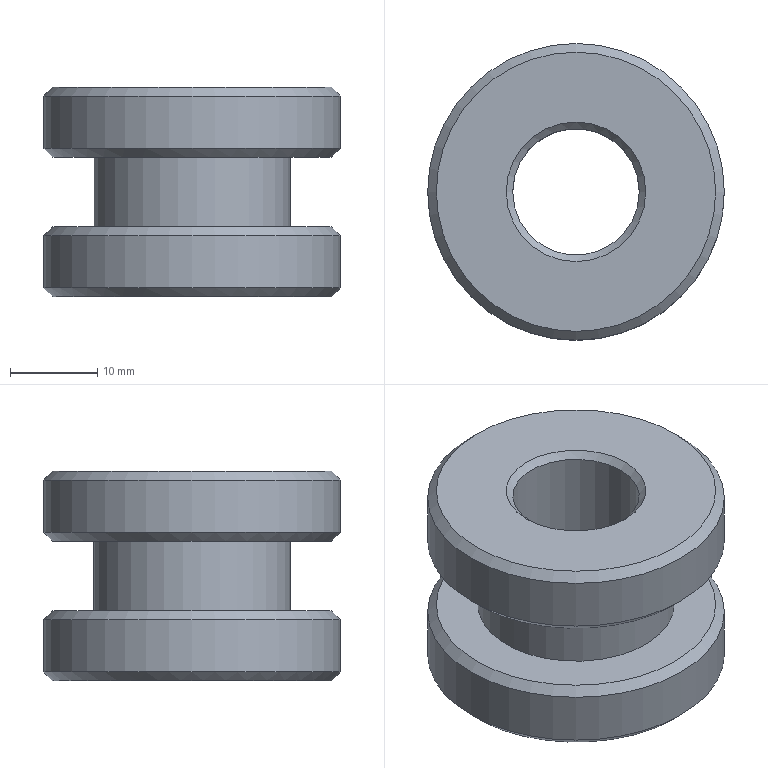Part | STEP file | YBQDJ-QD-9 | 1 solid | 14 faces | box 34 x 34 x 24 mm | volume 13509 mm3 | cone 6 | cylinder 4 | plane 4 | commonest cylinder face diameters 34 x2 14.5 x1 22.5 x1
STEP:
#1=CARTESIAN_POINT('',(0.,0.,0.));
#2=DIRECTION('',(0.,0.,1.));
#3=DIRECTION('',(1.,0.,0.));
#4=AXIS2_PLACEMENT_3D('',#1,#2,#3);
#5=CARTESIAN_POINT('',(-332.75,-195.,209.25));
#6=VERTEX_POINT('',#5);
#7=CARTESIAN_POINT('',(-340.,-195.,209.25));
#8=DIRECTION('',(0.,0.,-1.));
#9=DIRECTION('',(1.,0.,0.));
#10=AXIS2_PLACEMENT_3D('',#7,#8,#9);
#11=CIRCLE('',#10,7.25);
#12=CARTESIAN_POINT('',(-340.,-195.,232.5));
#13=DIRECTION('',(0.,0.,-1.));
#14=DIRECTION('',(-1.,0.,0.));
#15=AXIS2_PLACEMENT_3D('',#12,#13,#14);
#16=CYLINDRICAL_SURFACE('',#15,7.25);
#17=CARTESIAN_POINT('',(3.142,23.25));
#18=DIRECTION('',(1.,0.));
#19=VECTOR('',#18,1.);
#20=LINE('',#17,#19);
#21=(GEOMETRIC_REPRESENTATION_CONTEXT(2)PARAMETRIC_REPRESENTATION_CONTEXT()REPRESENTATION_CONTEXT('',''));
#22=DEFINITIONAL_REPRESENTATION('',(#20),#21);
#23=PCURVE('',#16,#22);
#24=CARTESIAN_POINT('',(-340.,-195.,209.25));
#25=DIRECTION('',(0.,0.,-1.));
#26=DIRECTION('',(-1.,0.,0.));
#27=AXIS2_PLACEMENT_3D('',#24,#25,#26);
#28=CONICAL_SURFACE('',#27,7.25,0.7854);
#29=CARTESIAN_POINT('',(3.142,0.));
#30=DIRECTION('',(1.,0.));
#31=VECTOR('',#30,1.);
#32=LINE('',#29,#31);
#33=(GEOMETRIC_REPRESENTATION_CONTEXT(2)PARAMETRIC_REPRESENTATION_CONTEXT()REPRESENTATION_CONTEXT('',''));
#34=DEFINITIONAL_REPRESENTATION('',(#32),#33);
#35=PCURVE('',#28,#34);
#36=SURFACE_CURVE('',#11,(#23,#35),.PCURVE_S1.);
#37=EDGE_CURVE('',#6,#6,#36,.T.);
#38=ORIENTED_EDGE('',*,*,#37,.F.);
#39=CARTESIAN_POINT('',(-332.75,-195.,231.75));
#40=VERTEX_POINT('',#39);
#41=CARTESIAN_POINT('',(-332.75,-195.,231.75));
#42=CARTESIAN_POINT('',(-332.75,-195.,209.25));
#43=B_SPLINE_CURVE_WITH_KNOTS('',1,(#41,#42),.UNSPECIFIED.,.F.,.F.,(2,2),(0.75,23.25),.PIECEWISE_BEZIER_KNOTS.);
#44=CARTESIAN_POINT('',(3.142,0.));
#45=DIRECTION('',(0.,1.));
#46=VECTOR('',#45,1.);
#47=LINE('',#44,#46);
#48=(GEOMETRIC_REPRESENTATION_CONTEXT(2)PARAMETRIC_REPRESENTATION_CONTEXT()REPRESENTATION_CONTEXT('',''));
#49=DEFINITIONAL_REPRESENTATION('',(#47),#48);
#50=PCURVE('',#16,#49);
#51=CARTESIAN_POINT('',(9.425,0.));
#52=DIRECTION('',(0.,1.));
#53=VECTOR('',#52,1.);
#54=LINE('',#51,#53);
#55=(GEOMETRIC_REPRESENTATION_CONTEXT(2)PARAMETRIC_REPRESENTATION_CONTEXT()REPRESENTATION_CONTEXT('',''));
#56=DEFINITIONAL_REPRESENTATION('',(#54),#55);
#57=PCURVE('',#16,#56);
#58=SEAM_CURVE('',#43,(#50,#57),.PCURVE_S1.);
#59=EDGE_CURVE('',#40,#6,#58,.T.);
#60=ORIENTED_EDGE('',*,*,#59,.F.);
#61=CARTESIAN_POINT('',(-340.,-195.,231.75));
#62=DIRECTION('',(0.,0.,1.));
#63=DIRECTION('',(1.,0.,0.));
#64=AXIS2_PLACEMENT_3D('',#61,#62,#63);
#65=CIRCLE('',#64,7.25);
#66=CARTESIAN_POINT('',(9.425,0.75));
#67=DIRECTION('',(-1.,0.));
#68=VECTOR('',#67,1.);
#69=LINE('',#66,#68);
#70=(GEOMETRIC_REPRESENTATION_CONTEXT(2)PARAMETRIC_REPRESENTATION_CONTEXT()REPRESENTATION_CONTEXT('',''));
#71=DEFINITIONAL_REPRESENTATION('',(#69),#70);
#72=PCURVE('',#16,#71);
#73=CARTESIAN_POINT('',(-340.,-195.,231.75));
#74=DIRECTION('',(0.,0.,1.));
#75=DIRECTION('',(1.,0.,0.));
#76=AXIS2_PLACEMENT_3D('',#73,#74,#75);
#77=CONICAL_SURFACE('',#76,7.25,0.7854);
#78=CARTESIAN_POINT('',(0.,0.));
#79=DIRECTION('',(1.,0.));
#80=VECTOR('',#79,1.);
#81=LINE('',#78,#80);
#82=(GEOMETRIC_REPRESENTATION_CONTEXT(2)PARAMETRIC_REPRESENTATION_CONTEXT()REPRESENTATION_CONTEXT('',''));
#83=DEFINITIONAL_REPRESENTATION('',(#81),#82);
#84=PCURVE('',#77,#83);
#85=SURFACE_CURVE('',#65,(#72,#84),.PCURVE_S1.);
#86=EDGE_CURVE('',#40,#40,#85,.T.);
#87=ORIENTED_EDGE('',*,*,#86,.F.);
#88=ORIENTED_EDGE('',*,*,#59,.T.);
#89=EDGE_LOOP('',(#38,#60,#87,#88));
#90=FACE_BOUND('',#89,.F.);
#91=ADVANCED_FACE('',(#90),#16,.F.);
#92=CARTESIAN_POINT('',(-323.,-195.,225.5));
#93=VERTEX_POINT('',#92);
#94=CARTESIAN_POINT('',(-357.,-195.,225.5));
#95=VERTEX_POINT('',#94);
#96=CARTESIAN_POINT('',(-340.,-195.,225.5));
#97=DIRECTION('',(0.,0.,1.));
#98=DIRECTION('',(1.,0.,0.));
#99=AXIS2_PLACEMENT_3D('',#96,#97,#98);
#100=CIRCLE('',#99,17.);
#101=CARTESIAN_POINT('',(-340.,-195.,232.5));
#102=DIRECTION('',(0.,0.,-1.));
#103=DIRECTION('',(-1.,0.,0.));
#104=AXIS2_PLACEMENT_3D('',#101,#102,#103);
#105=CYLINDRICAL_SURFACE('',#104,17.);
#106=CARTESIAN_POINT('',(3.142,7.));
#107=DIRECTION('',(-1.,0.));
#108=VECTOR('',#107,1.);
#109=LINE('',#106,#108);
#110=(GEOMETRIC_REPRESENTATION_CONTEXT(2)PARAMETRIC_REPRESENTATION_CONTEXT()REPRESENTATION_CONTEXT('',''));
#111=DEFINITIONAL_REPRESENTATION('',(#109),#110);
#112=PCURVE('',#105,#111);
#113=CARTESIAN_POINT('',(-340.,-195.,225.5));
#114=DIRECTION('',(0.,0.,1.));
#115=DIRECTION('',(1.,0.,0.));
#116=AXIS2_PLACEMENT_3D('',#113,#114,#115);
#117=CONICAL_SURFACE('',#116,17.,0.7854);
#118=CARTESIAN_POINT('',(0.,0.));
#119=DIRECTION('',(1.,0.));
#120=VECTOR('',#119,1.);
#121=LINE('',#118,#120);
#122=(GEOMETRIC_REPRESENTATION_CONTEXT(2)PARAMETRIC_REPRESENTATION_CONTEXT()REPRESENTATION_CONTEXT('',''));
#123=DEFINITIONAL_REPRESENTATION('',(#121),#122);
#124=PCURVE('',#117,#123);
#125=SURFACE_CURVE('',#100,(#112,#124),.PCURVE_S1.);
#126=EDGE_CURVE('',#93,#95,#125,.T.);
#127=ORIENTED_EDGE('',*,*,#126,.T.);
#128=CARTESIAN_POINT('',(-357.,-195.,231.5));
#129=VERTEX_POINT('',#128);
#130=CARTESIAN_POINT('',(-357.,-195.,231.5));
#131=CARTESIAN_POINT('',(-357.,-195.,225.5));
#132=B_SPLINE_CURVE_WITH_KNOTS('',1,(#130,#131),.UNSPECIFIED.,.F.,.F.,(2,2),(1.,7.),.PIECEWISE_BEZIER_KNOTS.);
#133=CARTESIAN_POINT('',(0.,0.));
#134=DIRECTION('',(0.,1.));
#135=VECTOR('',#134,1.);
#136=LINE('',#133,#135);
#137=(GEOMETRIC_REPRESENTATION_CONTEXT(2)PARAMETRIC_REPRESENTATION_CONTEXT()REPRESENTATION_CONTEXT('',''));
#138=DEFINITIONAL_REPRESENTATION('',(#136),#137);
#139=PCURVE('',#105,#138);
#140=CARTESIAN_POINT('',(6.283,0.));
#141=DIRECTION('',(0.,1.));
#142=VECTOR('',#141,1.);
#143=LINE('',#140,#142);
#144=(GEOMETRIC_REPRESENTATION_CONTEXT(2)PARAMETRIC_REPRESENTATION_CONTEXT()REPRESENTATION_CONTEXT('',''));
#145=DEFINITIONAL_REPRESENTATION('',(#143),#144);
#146=PCURVE('',#105,#145);
#147=SEAM_CURVE('',#132,(#139,#146),.PCURVE_S1.);
#148=EDGE_CURVE('',#129,#95,#147,.T.);
#149=ORIENTED_EDGE('',*,*,#148,.F.);
#150=CARTESIAN_POINT('',(-340.,-195.,231.5));
#151=DIRECTION('',(0.,0.,-1.));
#152=DIRECTION('',(-1.,0.,0.));
#153=AXIS2_PLACEMENT_3D('',#150,#151,#152);
#154=CIRCLE('',#153,17.);
#155=CARTESIAN_POINT('',(0.,1.));
#156=DIRECTION('',(1.,0.));
#157=VECTOR('',#156,1.);
#158=LINE('',#155,#157);
#159=(GEOMETRIC_REPRESENTATION_CONTEXT(2)PARAMETRIC_REPRESENTATION_CONTEXT()REPRESENTATION_CONTEXT('',''));
#160=DEFINITIONAL_REPRESENTATION('',(#158),#159);
#161=PCURVE('',#105,#160);
#162=CARTESIAN_POINT('',(-340.,-195.,232.5));
#163=DIRECTION('',(0.,0.,-1.));
#164=DIRECTION('',(-1.,0.,0.));
#165=AXIS2_PLACEMENT_3D('',#162,#163,#164);
#166=CONICAL_SURFACE('',#165,16.,0.7854);
#167=CARTESIAN_POINT('',(0.,1.));
#168=DIRECTION('',(1.,0.));
#169=VECTOR('',#168,1.);
#170=LINE('',#167,#169);
#171=(GEOMETRIC_REPRESENTATION_CONTEXT(2)PARAMETRIC_REPRESENTATION_CONTEXT()REPRESENTATION_CONTEXT('',''));
#172=DEFINITIONAL_REPRESENTATION('',(#170),#171);
#173=PCURVE('',#166,#172);
#174=SURFACE_CURVE('',#154,(#161,#173),.PCURVE_S1.);
#175=EDGE_CURVE('',#129,#129,#174,.T.);
#176=ORIENTED_EDGE('',*,*,#175,.T.);
#177=ORIENTED_EDGE('',*,*,#148,.T.);
#178=CARTESIAN_POINT('',(-340.,-195.,225.5));
#179=DIRECTION('',(0.,0.,1.));
#180=DIRECTION('',(1.,0.,0.));
#181=AXIS2_PLACEMENT_3D('',#178,#179,#180);
#182=CIRCLE('',#181,17.);
#183=CARTESIAN_POINT('',(9.425,7.));
#184=DIRECTION('',(-1.,0.));
#185=VECTOR('',#184,1.);
#186=LINE('',#183,#185);
#187=(GEOMETRIC_REPRESENTATION_CONTEXT(2)PARAMETRIC_REPRESENTATION_CONTEXT()REPRESENTATION_CONTEXT('',''));
#188=DEFINITIONAL_REPRESENTATION('',(#186),#187);
#189=PCURVE('',#105,#188);
#190=CARTESIAN_POINT('',(0.,0.));
#191=DIRECTION('',(1.,0.));
#192=VECTOR('',#191,1.);
#193=LINE('',#190,#192);
#194=(GEOMETRIC_REPRESENTATION_CONTEXT(2)PARAMETRIC_REPRESENTATION_CONTEXT()REPRESENTATION_CONTEXT('',''));
#195=DEFINITIONAL_REPRESENTATION('',(#193),#194);
#196=PCURVE('',#117,#195);
#197=SURFACE_CURVE('',#182,(#189,#196),.PCURVE_S1.);
#198=EDGE_CURVE('',#95,#93,#197,.T.);
#199=ORIENTED_EDGE('',*,*,#198,.T.);
#200=EDGE_LOOP('',(#127,#149,#176,#177,#199));
#201=FACE_BOUND('',#200,.T.);
#202=ADVANCED_FACE('',(#201),#105,.T.);
#203=CARTESIAN_POINT('',(-324.,-195.,232.5));
#204=VERTEX_POINT('',#203);
#205=CARTESIAN_POINT('',(-356.,-195.,232.5));
#206=VERTEX_POINT('',#205);
#207=CARTESIAN_POINT('',(-340.,-195.,232.5));
#208=DIRECTION('',(0.,0.,1.));
#209=DIRECTION('',(1.,0.,0.));
#210=AXIS2_PLACEMENT_3D('',#207,#208,#209);
#211=CIRCLE('',#210,16.);
#212=CARTESIAN_POINT('',(-340.,-195.,232.5));
#213=DIRECTION('',(0.,0.,1.));
#214=DIRECTION('',(1.,0.,0.));
#215=AXIS2_PLACEMENT_3D('',#212,#213,#214);
#216=PLANE('',#215);
#217=CARTESIAN_POINT('',(0.,0.));
#218=DIRECTION('',(1.,0.));
#219=AXIS2_PLACEMENT_2D('',#217,#218);
#220=CIRCLE('',#219,16.);
#221=(GEOMETRIC_REPRESENTATION_CONTEXT(2)PARAMETRIC_REPRESENTATION_CONTEXT()REPRESENTATION_CONTEXT('',''));
#222=DEFINITIONAL_REPRESENTATION('',(#220),#221);
#223=PCURVE('',#216,#222);
#224=CARTESIAN_POINT('',(3.142,0.));
#225=DIRECTION('',(-1.,0.));
#226=VECTOR('',#225,1.);
#227=LINE('',#224,#226);
#228=(GEOMETRIC_REPRESENTATION_CONTEXT(2)PARAMETRIC_REPRESENTATION_CONTEXT()REPRESENTATION_CONTEXT('',''));
#229=DEFINITIONAL_REPRESENTATION('',(#227),#228);
#230=PCURVE('',#166,#229);
#231=SURFACE_CURVE('',#211,(#223,#230),.PCURVE_S1.);
#232=EDGE_CURVE('',#204,#206,#231,.T.);
#233=ORIENTED_EDGE('',*,*,#232,.T.);
#234=CARTESIAN_POINT('',(-340.,-195.,232.5));
#235=DIRECTION('',(0.,0.,1.));
#236=DIRECTION('',(1.,0.,0.));
#237=AXIS2_PLACEMENT_3D('',#234,#235,#236);
#238=CIRCLE('',#237,16.);
#239=CARTESIAN_POINT('',(0.,0.));
#240=DIRECTION('',(1.,0.));
#241=AXIS2_PLACEMENT_2D('',#239,#240);
#242=CIRCLE('',#241,16.);
#243=(GEOMETRIC_REPRESENTATION_CONTEXT(2)PARAMETRIC_REPRESENTATION_CONTEXT()REPRESENTATION_CONTEXT('',''));
#244=DEFINITIONAL_REPRESENTATION('',(#242),#243);
#245=PCURVE('',#216,#244);
#246=CARTESIAN_POINT('',(9.425,0.));
#247=DIRECTION('',(-1.,0.));
#248=VECTOR('',#247,1.);
#249=LINE('',#246,#248);
#250=(GEOMETRIC_REPRESENTATION_CONTEXT(2)PARAMETRIC_REPRESENTATION_CONTEXT()REPRESENTATION_CONTEXT('',''));
#251=DEFINITIONAL_REPRESENTATION('',(#249),#250);
#252=PCURVE('',#166,#251);
#253=SURFACE_CURVE('',#238,(#245,#252),.PCURVE_S1.);
#254=EDGE_CURVE('',#206,#204,#253,.T.);
#255=ORIENTED_EDGE('',*,*,#254,.T.);
#256=EDGE_LOOP('',(#233,#255));
#257=FACE_BOUND('',#256,.T.);
#258=CARTESIAN_POINT('',(-332.,-195.,232.5));
#259=VERTEX_POINT('',#258);
#260=CARTESIAN_POINT('',(-340.,-195.,232.5));
#261=DIRECTION('',(0.,0.,-1.));
#262=DIRECTION('',(1.,0.,0.));
#263=AXIS2_PLACEMENT_3D('',#260,#261,#262);
#264=CIRCLE('',#263,8.);
#265=CARTESIAN_POINT('',(8.,0.));
#266=CARTESIAN_POINT('',(8.,-13.856));
#267=CARTESIAN_POINT('',(-4.,-6.928));
#268=CARTESIAN_POINT('',(-16.,0.));
#269=CARTESIAN_POINT('',(-4.,6.928));
#270=CARTESIAN_POINT('',(8.,13.856));
#271=CARTESIAN_POINT('',(8.,0.));
#272=(BOUNDED_CURVE()B_SPLINE_CURVE(2,(#265,#266,#267,#268,#269,#270,#271),.UNSPECIFIED.,.T.,.F.)B_SPLINE_CURVE_WITH_KNOTS((1,2,2,2,2,1),(-2.094,0.,2.094,4.189,6.283,8.378),.UNSPECIFIED.)CURVE()GEOMETRIC_REPRESENTATION_ITEM()RATIONAL_B_SPLINE_CURVE((1.,0.5,1.,0.5,1.,0.5,1.))REPRESENTATION_ITEM(''));
#273=(GEOMETRIC_REPRESENTATION_CONTEXT(2)PARAMETRIC_REPRESENTATION_CONTEXT()REPRESENTATION_CONTEXT('',''));
#274=DEFINITIONAL_REPRESENTATION('',(#272),#273);
#275=PCURVE('',#216,#274);
#276=CARTESIAN_POINT('',(6.283,0.75));
#277=DIRECTION('',(-1.,0.));
#278=VECTOR('',#277,1.);
#279=LINE('',#276,#278);
#280=(GEOMETRIC_REPRESENTATION_CONTEXT(2)PARAMETRIC_REPRESENTATION_CONTEXT()REPRESENTATION_CONTEXT('',''));
#281=DEFINITIONAL_REPRESENTATION('',(#279),#280);
#282=PCURVE('',#77,#281);
#283=SURFACE_CURVE('',#264,(#275,#282),.PCURVE_S1.);
#284=EDGE_CURVE('',#259,#259,#283,.T.);
#285=ORIENTED_EDGE('',*,*,#284,.T.);
#286=EDGE_LOOP('',(#285));
#287=FACE_BOUND('',#286,.T.);
#288=ADVANCED_FACE('',(#257,#287),#216,.T.);
#289=CARTESIAN_POINT('',(-324.,-195.,224.5));
#290=VERTEX_POINT('',#289);
#291=CARTESIAN_POINT('',(-340.,-195.,224.5));
#292=DIRECTION('',(0.,0.,-1.));
#293=DIRECTION('',(1.,0.,0.));
#294=AXIS2_PLACEMENT_3D('',#291,#292,#293);
#295=CIRCLE('',#294,16.);
#296=CARTESIAN_POINT('',(-340.,-195.,224.5));
#297=DIRECTION('',(0.,0.,1.));
#298=DIRECTION('',(1.,0.,0.));
#299=AXIS2_PLACEMENT_3D('',#296,#297,#298);
#300=PLANE('',#299);
#301=CARTESIAN_POINT('',(16.,0.));
#302=CARTESIAN_POINT('',(16.,-27.713));
#303=CARTESIAN_POINT('',(-8.,-13.856));
#304=CARTESIAN_POINT('',(-32.,0.));
#305=CARTESIAN_POINT('',(-8.,13.856));
#306=CARTESIAN_POINT('',(16.,27.713));
#307=CARTESIAN_POINT('',(16.,0.));
#308=(BOUNDED_CURVE()B_SPLINE_CURVE(2,(#301,#302,#303,#304,#305,#306,#307),.UNSPECIFIED.,.T.,.F.)B_SPLINE_CURVE_WITH_KNOTS((1,2,2,2,2,1),(-2.094,0.,2.094,4.189,6.283,8.378),.UNSPECIFIED.)CURVE()GEOMETRIC_REPRESENTATION_ITEM()RATIONAL_B_SPLINE_CURVE((1.,0.5,1.,0.5,1.,0.5,1.))REPRESENTATION_ITEM(''));
#309=(GEOMETRIC_REPRESENTATION_CONTEXT(2)PARAMETRIC_REPRESENTATION_CONTEXT()REPRESENTATION_CONTEXT('',''));
#310=DEFINITIONAL_REPRESENTATION('',(#308),#309);
#311=PCURVE('',#300,#310);
#312=CARTESIAN_POINT('',(6.283,-1.));
#313=DIRECTION('',(-1.,0.));
#314=VECTOR('',#313,1.);
#315=LINE('',#312,#314);
#316=(GEOMETRIC_REPRESENTATION_CONTEXT(2)PARAMETRIC_REPRESENTATION_CONTEXT()REPRESENTATION_CONTEXT('',''));
#317=DEFINITIONAL_REPRESENTATION('',(#315),#316);
#318=PCURVE('',#117,#317);
#319=SURFACE_CURVE('',#295,(#311,#318),.PCURVE_S1.);
#320=EDGE_CURVE('',#290,#290,#319,.T.);
#321=ORIENTED_EDGE('',*,*,#320,.T.);
#322=EDGE_LOOP('',(#321));
#323=FACE_BOUND('',#322,.T.);
#324=CARTESIAN_POINT('',(-328.75,-195.,224.5));
#325=VERTEX_POINT('',#324);
#326=CARTESIAN_POINT('',(-340.,-195.,224.5));
#327=DIRECTION('',(0.,0.,1.));
#328=DIRECTION('',(1.,0.,0.));
#329=AXIS2_PLACEMENT_3D('',#326,#327,#328);
#330=CIRCLE('',#329,11.25);
#331=CARTESIAN_POINT('',(0.,0.));
#332=DIRECTION('',(1.,0.));
#333=AXIS2_PLACEMENT_2D('',#331,#332);
#334=CIRCLE('',#333,11.25);
#335=(GEOMETRIC_REPRESENTATION_CONTEXT(2)PARAMETRIC_REPRESENTATION_CONTEXT()REPRESENTATION_CONTEXT('',''));
#336=DEFINITIONAL_REPRESENTATION('',(#334),#335);
#337=PCURVE('',#300,#336);
#338=CARTESIAN_POINT('',(-340.,-195.,224.5));
#339=DIRECTION('',(0.,0.,-1.));
#340=DIRECTION('',(-1.,0.,0.));
#341=AXIS2_PLACEMENT_3D('',#338,#339,#340);
#342=CYLINDRICAL_SURFACE('',#341,11.25);
#343=CARTESIAN_POINT('',(9.425,0.));
#344=DIRECTION('',(-1.,0.));
#345=VECTOR('',#344,1.);
#346=LINE('',#343,#345);
#347=(GEOMETRIC_REPRESENTATION_CONTEXT(2)PARAMETRIC_REPRESENTATION_CONTEXT()REPRESENTATION_CONTEXT('',''));
#348=DEFINITIONAL_REPRESENTATION('',(#346),#347);
#349=PCURVE('',#342,#348);
#350=SURFACE_CURVE('',#330,(#337,#349),.PCURVE_S1.);
#351=EDGE_CURVE('',#325,#325,#350,.T.);
#352=ORIENTED_EDGE('',*,*,#351,.T.);
#353=EDGE_LOOP('',(#352));
#354=FACE_BOUND('',#353,.T.);
#355=ADVANCED_FACE('',(#323,#354),#300,.F.);
#356=CARTESIAN_POINT('',(-323.,-195.,209.5));
#357=VERTEX_POINT('',#356);
#358=CARTESIAN_POINT('',(-357.,-195.,209.5));
#359=VERTEX_POINT('',#358);
#360=CARTESIAN_POINT('',(-340.,-195.,209.5));
#361=DIRECTION('',(0.,0.,1.));
#362=DIRECTION('',(1.,0.,0.));
#363=AXIS2_PLACEMENT_3D('',#360,#361,#362);
#364=CIRCLE('',#363,17.);
#365=CARTESIAN_POINT('',(-340.,-195.,216.5));
#366=DIRECTION('',(0.,0.,-1.));
#367=DIRECTION('',(-1.,0.,0.));
#368=AXIS2_PLACEMENT_3D('',#365,#366,#367);
#369=CYLINDRICAL_SURFACE('',#368,17.);
#370=CARTESIAN_POINT('',(3.142,7.));
#371=DIRECTION('',(-1.,0.));
#372=VECTOR('',#371,1.);
#373=LINE('',#370,#372);
#374=(GEOMETRIC_REPRESENTATION_CONTEXT(2)PARAMETRIC_REPRESENTATION_CONTEXT()REPRESENTATION_CONTEXT('',''));
#375=DEFINITIONAL_REPRESENTATION('',(#373),#374);
#376=PCURVE('',#369,#375);
#377=CARTESIAN_POINT('',(-340.,-195.,209.5));
#378=DIRECTION('',(0.,0.,1.));
#379=DIRECTION('',(1.,0.,0.));
#380=AXIS2_PLACEMENT_3D('',#377,#378,#379);
#381=CONICAL_SURFACE('',#380,17.,0.7854);
#382=CARTESIAN_POINT('',(0.,0.));
#383=DIRECTION('',(1.,0.));
#384=VECTOR('',#383,1.);
#385=LINE('',#382,#384);
#386=(GEOMETRIC_REPRESENTATION_CONTEXT(2)PARAMETRIC_REPRESENTATION_CONTEXT()REPRESENTATION_CONTEXT('',''));
#387=DEFINITIONAL_REPRESENTATION('',(#385),#386);
#388=PCURVE('',#381,#387);
#389=SURFACE_CURVE('',#364,(#376,#388),.PCURVE_S1.);
#390=EDGE_CURVE('',#357,#359,#389,.T.);
#391=ORIENTED_EDGE('',*,*,#390,.T.);
#392=CARTESIAN_POINT('',(-357.,-195.,215.5));
#393=VERTEX_POINT('',#392);
#394=CARTESIAN_POINT('',(-357.,-195.,215.5));
#395=CARTESIAN_POINT('',(-357.,-195.,209.5));
#396=B_SPLINE_CURVE_WITH_KNOTS('',1,(#394,#395),.UNSPECIFIED.,.F.,.F.,(2,2),(1.,7.),.PIECEWISE_BEZIER_KNOTS.);
#397=CARTESIAN_POINT('',(0.,0.));
#398=DIRECTION('',(0.,1.));
#399=VECTOR('',#398,1.);
#400=LINE('',#397,#399);
#401=(GEOMETRIC_REPRESENTATION_CONTEXT(2)PARAMETRIC_REPRESENTATION_CONTEXT()REPRESENTATION_CONTEXT('',''));
#402=DEFINITIONAL_REPRESENTATION('',(#400),#401);
#403=PCURVE('',#369,#402);
#404=CARTESIAN_POINT('',(6.283,0.));
#405=DIRECTION('',(0.,1.));
#406=VECTOR('',#405,1.);
#407=LINE('',#404,#406);
#408=(GEOMETRIC_REPRESENTATION_CONTEXT(2)PARAMETRIC_REPRESENTATION_CONTEXT()REPRESENTATION_CONTEXT('',''));
#409=DEFINITIONAL_REPRESENTATION('',(#407),#408);
#410=PCURVE('',#369,#409);
#411=SEAM_CURVE('',#396,(#403,#410),.PCURVE_S1.);
#412=EDGE_CURVE('',#393,#359,#411,.T.);
#413=ORIENTED_EDGE('',*,*,#412,.F.);
#414=CARTESIAN_POINT('',(-340.,-195.,215.5));
#415=DIRECTION('',(0.,0.,-1.));
#416=DIRECTION('',(-1.,0.,0.));
#417=AXIS2_PLACEMENT_3D('',#414,#415,#416);
#418=CIRCLE('',#417,17.);
#419=CARTESIAN_POINT('',(0.,1.));
#420=DIRECTION('',(1.,0.));
#421=VECTOR('',#420,1.);
#422=LINE('',#419,#421);
#423=(GEOMETRIC_REPRESENTATION_CONTEXT(2)PARAMETRIC_REPRESENTATION_CONTEXT()REPRESENTATION_CONTEXT('',''));
#424=DEFINITIONAL_REPRESENTATION('',(#422),#423);
#425=PCURVE('',#369,#424);
#426=CARTESIAN_POINT('',(-340.,-195.,216.5));
#427=DIRECTION('',(0.,0.,-1.));
#428=DIRECTION('',(-1.,0.,0.));
#429=AXIS2_PLACEMENT_3D('',#426,#427,#428);
#430=CONICAL_SURFACE('',#429,16.,0.7854);
#431=CARTESIAN_POINT('',(0.,1.));
#432=DIRECTION('',(1.,0.));
#433=VECTOR('',#432,1.);
#434=LINE('',#431,#433);
#435=(GEOMETRIC_REPRESENTATION_CONTEXT(2)PARAMETRIC_REPRESENTATION_CONTEXT()REPRESENTATION_CONTEXT('',''));
#436=DEFINITIONAL_REPRESENTATION('',(#434),#435);
#437=PCURVE('',#430,#436);
#438=SURFACE_CURVE('',#418,(#425,#437),.PCURVE_S1.);
#439=EDGE_CURVE('',#393,#393,#438,.T.);
#440=ORIENTED_EDGE('',*,*,#439,.T.);
#441=ORIENTED_EDGE('',*,*,#412,.T.);
#442=CARTESIAN_POINT('',(-340.,-195.,209.5));
#443=DIRECTION('',(0.,0.,1.));
#444=DIRECTION('',(1.,0.,0.));
#445=AXIS2_PLACEMENT_3D('',#442,#443,#444);
#446=CIRCLE('',#445,17.);
#447=CARTESIAN_POINT('',(9.425,7.));
#448=DIRECTION('',(-1.,0.));
#449=VECTOR('',#448,1.);
#450=LINE('',#447,#449);
#451=(GEOMETRIC_REPRESENTATION_CONTEXT(2)PARAMETRIC_REPRESENTATION_CONTEXT()REPRESENTATION_CONTEXT('',''));
#452=DEFINITIONAL_REPRESENTATION('',(#450),#451);
#453=PCURVE('',#369,#452);
#454=CARTESIAN_POINT('',(0.,0.));
#455=DIRECTION('',(1.,0.));
#456=VECTOR('',#455,1.);
#457=LINE('',#454,#456);
#458=(GEOMETRIC_REPRESENTATION_CONTEXT(2)PARAMETRIC_REPRESENTATION_CONTEXT()REPRESENTATION_CONTEXT('',''));
#459=DEFINITIONAL_REPRESENTATION('',(#457),#458);
#460=PCURVE('',#381,#459);
#461=SURFACE_CURVE('',#446,(#453,#460),.PCURVE_S1.);
#462=EDGE_CURVE('',#359,#357,#461,.T.);
#463=ORIENTED_EDGE('',*,*,#462,.T.);
#464=EDGE_LOOP('',(#391,#413,#440,#441,#463));
#465=FACE_BOUND('',#464,.T.);
#466=ADVANCED_FACE('',(#465),#369,.T.);
#467=CARTESIAN_POINT('',(-324.,-195.,216.5));
#468=VERTEX_POINT('',#467);
#469=CARTESIAN_POINT('',(-356.,-195.,216.5));
#470=VERTEX_POINT('',#469);
#471=CARTESIAN_POINT('',(-340.,-195.,216.5));
#472=DIRECTION('',(0.,0.,1.));
#473=DIRECTION('',(1.,0.,0.));
#474=AXIS2_PLACEMENT_3D('',#471,#472,#473);
#475=CIRCLE('',#474,16.);
#476=CARTESIAN_POINT('',(-340.,-195.,216.5));
#477=DIRECTION('',(0.,0.,1.));
#478=DIRECTION('',(1.,0.,0.));
#479=AXIS2_PLACEMENT_3D('',#476,#477,#478);
#480=PLANE('',#479);
#481=CARTESIAN_POINT('',(0.,0.));
#482=DIRECTION('',(1.,0.));
#483=AXIS2_PLACEMENT_2D('',#481,#482);
#484=CIRCLE('',#483,16.);
#485=(GEOMETRIC_REPRESENTATION_CONTEXT(2)PARAMETRIC_REPRESENTATION_CONTEXT()REPRESENTATION_CONTEXT('',''));
#486=DEFINITIONAL_REPRESENTATION('',(#484),#485);
#487=PCURVE('',#480,#486);
#488=CARTESIAN_POINT('',(3.142,0.));
#489=DIRECTION('',(-1.,0.));
#490=VECTOR('',#489,1.);
#491=LINE('',#488,#490);
#492=(GEOMETRIC_REPRESENTATION_CONTEXT(2)PARAMETRIC_REPRESENTATION_CONTEXT()REPRESENTATION_CONTEXT('',''));
#493=DEFINITIONAL_REPRESENTATION('',(#491),#492);
#494=PCURVE('',#430,#493);
#495=SURFACE_CURVE('',#475,(#487,#494),.PCURVE_S1.);
#496=EDGE_CURVE('',#468,#470,#495,.T.);
#497=ORIENTED_EDGE('',*,*,#496,.T.);
#498=CARTESIAN_POINT('',(-340.,-195.,216.5));
#499=DIRECTION('',(0.,0.,1.));
#500=DIRECTION('',(1.,0.,0.));
#501=AXIS2_PLACEMENT_3D('',#498,#499,#500);
#502=CIRCLE('',#501,16.);
#503=CARTESIAN_POINT('',(0.,0.));
#504=DIRECTION('',(1.,0.));
#505=AXIS2_PLACEMENT_2D('',#503,#504);
#506=CIRCLE('',#505,16.);
#507=(GEOMETRIC_REPRESENTATION_CONTEXT(2)PARAMETRIC_REPRESENTATION_CONTEXT()REPRESENTATION_CONTEXT('',''));
#508=DEFINITIONAL_REPRESENTATION('',(#506),#507);
#509=PCURVE('',#480,#508);
#510=CARTESIAN_POINT('',(9.425,0.));
#511=DIRECTION('',(-1.,0.));
#512=VECTOR('',#511,1.);
#513=LINE('',#510,#512);
#514=(GEOMETRIC_REPRESENTATION_CONTEXT(2)PARAMETRIC_REPRESENTATION_CONTEXT()REPRESENTATION_CONTEXT('',''));
#515=DEFINITIONAL_REPRESENTATION('',(#513),#514);
#516=PCURVE('',#430,#515);
#517=SURFACE_CURVE('',#502,(#509,#516),.PCURVE_S1.);
#518=EDGE_CURVE('',#470,#468,#517,.T.);
#519=ORIENTED_EDGE('',*,*,#518,.T.);
#520=EDGE_LOOP('',(#497,#519));
#521=FACE_BOUND('',#520,.T.);
#522=CARTESIAN_POINT('',(-328.75,-195.,216.5));
#523=VERTEX_POINT('',#522);
#524=CARTESIAN_POINT('',(-340.,-195.,216.5));
#525=DIRECTION('',(0.,0.,1.));
#526=DIRECTION('',(1.,0.,0.));
#527=AXIS2_PLACEMENT_3D('',#524,#525,#526);
#528=CIRCLE('',#527,11.25);
#529=CARTESIAN_POINT('',(0.,0.));
#530=DIRECTION('',(1.,0.));
#531=AXIS2_PLACEMENT_2D('',#529,#530);
#532=CIRCLE('',#531,11.25);
#533=(GEOMETRIC_REPRESENTATION_CONTEXT(2)PARAMETRIC_REPRESENTATION_CONTEXT()REPRESENTATION_CONTEXT('',''));
#534=DEFINITIONAL_REPRESENTATION('',(#532),#533);
#535=PCURVE('',#480,#534);
#536=CARTESIAN_POINT('',(9.425,8.));
#537=DIRECTION('',(-1.,0.));
#538=VECTOR('',#537,1.);
#539=LINE('',#536,#538);
#540=(GEOMETRIC_REPRESENTATION_CONTEXT(2)PARAMETRIC_REPRESENTATION_CONTEXT()REPRESENTATION_CONTEXT('',''));
#541=DEFINITIONAL_REPRESENTATION('',(#539),#540);
#542=PCURVE('',#342,#541);
#543=SURFACE_CURVE('',#528,(#535,#542),.PCURVE_S1.);
#544=EDGE_CURVE('',#523,#523,#543,.T.);
#545=ORIENTED_EDGE('',*,*,#544,.F.);
#546=EDGE_LOOP('',(#545));
#547=FACE_BOUND('',#546,.T.);
#548=ADVANCED_FACE('',(#521,#547),#480,.T.);
#549=CARTESIAN_POINT('',(-324.,-195.,208.5));
#550=VERTEX_POINT('',#549);
#551=CARTESIAN_POINT('',(-340.,-195.,208.5));
#552=DIRECTION('',(0.,0.,-1.));
#553=DIRECTION('',(1.,0.,0.));
#554=AXIS2_PLACEMENT_3D('',#551,#552,#553);
#555=CIRCLE('',#554,16.);
#556=CARTESIAN_POINT('',(-340.,-195.,208.5));
#557=DIRECTION('',(0.,0.,1.));
#558=DIRECTION('',(1.,0.,0.));
#559=AXIS2_PLACEMENT_3D('',#556,#557,#558);
#560=PLANE('',#559);
#561=CARTESIAN_POINT('',(16.,0.));
#562=CARTESIAN_POINT('',(16.,-27.713));
#563=CARTESIAN_POINT('',(-8.,-13.856));
#564=CARTESIAN_POINT('',(-32.,0.));
#565=CARTESIAN_POINT('',(-8.,13.856));
#566=CARTESIAN_POINT('',(16.,27.713));
#567=CARTESIAN_POINT('',(16.,0.));
#568=(BOUNDED_CURVE()B_SPLINE_CURVE(2,(#561,#562,#563,#564,#565,#566,#567),.UNSPECIFIED.,.T.,.F.)B_SPLINE_CURVE_WITH_KNOTS((1,2,2,2,2,1),(-2.094,0.,2.094,4.189,6.283,8.378),.UNSPECIFIED.)CURVE()GEOMETRIC_REPRESENTATION_ITEM()RATIONAL_B_SPLINE_CURVE((1.,0.5,1.,0.5,1.,0.5,1.))REPRESENTATION_ITEM(''));
#569=(GEOMETRIC_REPRESENTATION_CONTEXT(2)PARAMETRIC_REPRESENTATION_CONTEXT()REPRESENTATION_CONTEXT('',''));
#570=DEFINITIONAL_REPRESENTATION('',(#568),#569);
#571=PCURVE('',#560,#570);
#572=CARTESIAN_POINT('',(6.283,-1.));
#573=DIRECTION('',(-1.,0.));
#574=VECTOR('',#573,1.);
#575=LINE('',#572,#574);
#576=(GEOMETRIC_REPRESENTATION_CONTEXT(2)PARAMETRIC_REPRESENTATION_CONTEXT()REPRESENTATION_CONTEXT('',''));
#577=DEFINITIONAL_REPRESENTATION('',(#575),#576);
#578=PCURVE('',#381,#577);
#579=SURFACE_CURVE('',#555,(#571,#578),.PCURVE_S1.);
#580=EDGE_CURVE('',#550,#550,#579,.T.);
#581=ORIENTED_EDGE('',*,*,#580,.T.);
#582=EDGE_LOOP('',(#581));
#583=FACE_BOUND('',#582,.T.);
#584=CARTESIAN_POINT('',(-332.,-195.,208.5));
#585=VERTEX_POINT('',#584);
#586=CARTESIAN_POINT('',(-340.,-195.,208.5));
#587=DIRECTION('',(0.,0.,1.));
#588=DIRECTION('',(1.,0.,0.));
#589=AXIS2_PLACEMENT_3D('',#586,#587,#588);
#590=CIRCLE('',#589,8.);
#591=CARTESIAN_POINT('',(0.,0.));
#592=DIRECTION('',(1.,0.));
#593=AXIS2_PLACEMENT_2D('',#591,#592);
#594=CIRCLE('',#593,8.);
#595=(GEOMETRIC_REPRESENTATION_CONTEXT(2)PARAMETRIC_REPRESENTATION_CONTEXT()REPRESENTATION_CONTEXT('',''));
#596=DEFINITIONAL_REPRESENTATION('',(#594),#595);
#597=PCURVE('',#560,#596);
#598=CARTESIAN_POINT('',(9.425,0.75));
#599=DIRECTION('',(-1.,0.));
#600=VECTOR('',#599,1.);
#601=LINE('',#598,#600);
#602=(GEOMETRIC_REPRESENTATION_CONTEXT(2)PARAMETRIC_REPRESENTATION_CONTEXT()REPRESENTATION_CONTEXT('',''));
#603=DEFINITIONAL_REPRESENTATION('',(#601),#602);
#604=PCURVE('',#28,#603);
#605=SURFACE_CURVE('',#590,(#597,#604),.PCURVE_S1.);
#606=EDGE_CURVE('',#585,#585,#605,.T.);
#607=ORIENTED_EDGE('',*,*,#606,.T.);
#608=EDGE_LOOP('',(#607));
#609=FACE_BOUND('',#608,.T.);
#610=ADVANCED_FACE('',(#583,#609),#560,.F.);
#611=ORIENTED_EDGE('',*,*,#351,.F.);
#612=CARTESIAN_POINT('',(-328.75,-195.,224.5));
#613=CARTESIAN_POINT('',(-328.75,-195.,216.5));
#614=B_SPLINE_CURVE_WITH_KNOTS('',1,(#612,#613),.UNSPECIFIED.,.F.,.F.,(2,2),(0.,8.),.PIECEWISE_BEZIER_KNOTS.);
#615=CARTESIAN_POINT('',(9.425,0.));
#616=DIRECTION('',(0.,1.));
#617=VECTOR('',#616,1.);
#618=LINE('',#615,#617);
#619=(GEOMETRIC_REPRESENTATION_CONTEXT(2)PARAMETRIC_REPRESENTATION_CONTEXT()REPRESENTATION_CONTEXT('',''));
#620=DEFINITIONAL_REPRESENTATION('',(#618),#619);
#621=PCURVE('',#342,#620);
#622=CARTESIAN_POINT('',(3.142,0.));
#623=DIRECTION('',(0.,1.));
#624=VECTOR('',#623,1.);
#625=LINE('',#622,#624);
#626=(GEOMETRIC_REPRESENTATION_CONTEXT(2)PARAMETRIC_REPRESENTATION_CONTEXT()REPRESENTATION_CONTEXT('',''));
#627=DEFINITIONAL_REPRESENTATION('',(#625),#626);
#628=PCURVE('',#342,#627);
#629=SEAM_CURVE('',#614,(#621,#628),.PCURVE_S1.);
#630=EDGE_CURVE('',#325,#523,#629,.T.);
#631=ORIENTED_EDGE('',*,*,#630,.T.);
#632=ORIENTED_EDGE('',*,*,#544,.T.);
#633=ORIENTED_EDGE('',*,*,#630,.F.);
#634=EDGE_LOOP('',(#611,#631,#632,#633));
#635=FACE_BOUND('',#634,.T.);
#636=ADVANCED_FACE('',(#635),#342,.T.);
#637=ORIENTED_EDGE('',*,*,#606,.T.);
#638=CARTESIAN_POINT('',(-332.75,-195.,209.25));
#639=CARTESIAN_POINT('',(-332.,-195.,208.5));
#640=B_SPLINE_CURVE_WITH_KNOTS('',1,(#638,#639),.UNSPECIFIED.,.F.,.F.,(2,2),(0.,1.061),.PIECEWISE_BEZIER_KNOTS.);
#641=CARTESIAN_POINT('',(3.142,0.));
#642=DIRECTION('',(0.,1.));
#643=VECTOR('',#642,1.);
#644=LINE('',#641,#643);
#645=(GEOMETRIC_REPRESENTATION_CONTEXT(2)PARAMETRIC_REPRESENTATION_CONTEXT()REPRESENTATION_CONTEXT('',''));
#646=DEFINITIONAL_REPRESENTATION('',(#644),#645);
#647=PCURVE('',#28,#646);
#648=CARTESIAN_POINT('',(9.425,0.));
#649=DIRECTION('',(0.,1.));
#650=VECTOR('',#649,1.);
#651=LINE('',#648,#650);
#652=(GEOMETRIC_REPRESENTATION_CONTEXT(2)PARAMETRIC_REPRESENTATION_CONTEXT()REPRESENTATION_CONTEXT('',''));
#653=DEFINITIONAL_REPRESENTATION('',(#651),#652);
#654=PCURVE('',#28,#653);
#655=SEAM_CURVE('',#640,(#647,#654),.PCURVE_S1.);
#656=EDGE_CURVE('',#6,#585,#655,.T.);
#657=ORIENTED_EDGE('',*,*,#656,.F.);
#658=ORIENTED_EDGE('',*,*,#37,.T.);
#659=ORIENTED_EDGE('',*,*,#656,.T.);
#660=EDGE_LOOP('',(#637,#657,#658,#659));
#661=FACE_BOUND('',#660,.F.);
#662=ADVANCED_FACE('',(#661),#28,.F.);
#663=ORIENTED_EDGE('',*,*,#284,.T.);
#664=CARTESIAN_POINT('',(-332.75,-195.,231.75));
#665=CARTESIAN_POINT('',(-332.,-195.,232.5));
#666=B_SPLINE_CURVE_WITH_KNOTS('',1,(#664,#665),.UNSPECIFIED.,.F.,.F.,(2,2),(0.,1.061),.PIECEWISE_BEZIER_KNOTS.);
#667=CARTESIAN_POINT('',(0.,0.));
#668=DIRECTION('',(0.,1.));
#669=VECTOR('',#668,1.);
#670=LINE('',#667,#669);
#671=(GEOMETRIC_REPRESENTATION_CONTEXT(2)PARAMETRIC_REPRESENTATION_CONTEXT()REPRESENTATION_CONTEXT('',''));
#672=DEFINITIONAL_REPRESENTATION('',(#670),#671);
#673=PCURVE('',#77,#672);
#674=CARTESIAN_POINT('',(6.283,0.));
#675=DIRECTION('',(0.,1.));
#676=VECTOR('',#675,1.);
#677=LINE('',#674,#676);
#678=(GEOMETRIC_REPRESENTATION_CONTEXT(2)PARAMETRIC_REPRESENTATION_CONTEXT()REPRESENTATION_CONTEXT('',''));
#679=DEFINITIONAL_REPRESENTATION('',(#677),#678);
#680=PCURVE('',#77,#679);
#681=SEAM_CURVE('',#666,(#673,#680),.PCURVE_S1.);
#682=EDGE_CURVE('',#40,#259,#681,.T.);
#683=ORIENTED_EDGE('',*,*,#682,.F.);
#684=ORIENTED_EDGE('',*,*,#86,.T.);
#685=ORIENTED_EDGE('',*,*,#682,.T.);
#686=EDGE_LOOP('',(#663,#683,#684,#685));
#687=FACE_BOUND('',#686,.F.);
#688=ADVANCED_FACE('',(#687),#77,.F.);
#689=ORIENTED_EDGE('',*,*,#580,.F.);
#690=CARTESIAN_POINT('',(-324.,-195.,208.5));
#691=CARTESIAN_POINT('',(-323.,-195.,209.5));
#692=B_SPLINE_CURVE_WITH_KNOTS('',1,(#690,#691),.UNSPECIFIED.,.F.,.F.,(2,2),(-1.414,0.),.PIECEWISE_BEZIER_KNOTS.);
#693=CARTESIAN_POINT('',(6.283,0.));
#694=DIRECTION('',(0.,1.));
#695=VECTOR('',#694,1.);
#696=LINE('',#693,#695);
#697=(GEOMETRIC_REPRESENTATION_CONTEXT(2)PARAMETRIC_REPRESENTATION_CONTEXT()REPRESENTATION_CONTEXT('',''));
#698=DEFINITIONAL_REPRESENTATION('',(#696),#697);
#699=PCURVE('',#381,#698);
#700=CARTESIAN_POINT('',(0.,0.));
#701=DIRECTION('',(0.,1.));
#702=VECTOR('',#701,1.);
#703=LINE('',#700,#702);
#704=(GEOMETRIC_REPRESENTATION_CONTEXT(2)PARAMETRIC_REPRESENTATION_CONTEXT()REPRESENTATION_CONTEXT('',''));
#705=DEFINITIONAL_REPRESENTATION('',(#703),#704);
#706=PCURVE('',#381,#705);
#707=SEAM_CURVE('',#692,(#699,#706),.PCURVE_S1.);
#708=EDGE_CURVE('',#550,#357,#707,.T.);
#709=ORIENTED_EDGE('',*,*,#708,.T.);
#710=ORIENTED_EDGE('',*,*,#462,.F.);
#711=ORIENTED_EDGE('',*,*,#390,.F.);
#712=ORIENTED_EDGE('',*,*,#708,.F.);
#713=EDGE_LOOP('',(#689,#709,#710,#711,#712));
#714=FACE_BOUND('',#713,.T.);
#715=ADVANCED_FACE('',(#714),#381,.T.);
#716=ORIENTED_EDGE('',*,*,#439,.F.);
#717=CARTESIAN_POINT('',(-356.,-195.,216.5));
#718=CARTESIAN_POINT('',(-357.,-195.,215.5));
#719=B_SPLINE_CURVE_WITH_KNOTS('',1,(#717,#718),.UNSPECIFIED.,.F.,.F.,(2,2),(0.,1.414),.PIECEWISE_BEZIER_KNOTS.);
#720=CARTESIAN_POINT('',(0.,0.));
#721=DIRECTION('',(0.,1.));
#722=VECTOR('',#721,1.);
#723=LINE('',#720,#722);
#724=(GEOMETRIC_REPRESENTATION_CONTEXT(2)PARAMETRIC_REPRESENTATION_CONTEXT()REPRESENTATION_CONTEXT('',''));
#725=DEFINITIONAL_REPRESENTATION('',(#723),#724);
#726=PCURVE('',#430,#725);
#727=CARTESIAN_POINT('',(6.283,0.));
#728=DIRECTION('',(0.,1.));
#729=VECTOR('',#728,1.);
#730=LINE('',#727,#729);
#731=(GEOMETRIC_REPRESENTATION_CONTEXT(2)PARAMETRIC_REPRESENTATION_CONTEXT()REPRESENTATION_CONTEXT('',''));
#732=DEFINITIONAL_REPRESENTATION('',(#730),#731);
#733=PCURVE('',#430,#732);
#734=SEAM_CURVE('',#719,(#726,#733),.PCURVE_S1.);
#735=EDGE_CURVE('',#470,#393,#734,.T.);
#736=ORIENTED_EDGE('',*,*,#735,.F.);
#737=ORIENTED_EDGE('',*,*,#496,.F.);
#738=ORIENTED_EDGE('',*,*,#518,.F.);
#739=ORIENTED_EDGE('',*,*,#735,.T.);
#740=EDGE_LOOP('',(#716,#736,#737,#738,#739));
#741=FACE_BOUND('',#740,.T.);
#742=ADVANCED_FACE('',(#741),#430,.T.);
#743=ORIENTED_EDGE('',*,*,#320,.F.);
#744=CARTESIAN_POINT('',(-324.,-195.,224.5));
#745=CARTESIAN_POINT('',(-323.,-195.,225.5));
#746=B_SPLINE_CURVE_WITH_KNOTS('',1,(#744,#745),.UNSPECIFIED.,.F.,.F.,(2,2),(-1.414,0.),.PIECEWISE_BEZIER_KNOTS.);
#747=CARTESIAN_POINT('',(6.283,0.));
#748=DIRECTION('',(0.,1.));
#749=VECTOR('',#748,1.);
#750=LINE('',#747,#749);
#751=(GEOMETRIC_REPRESENTATION_CONTEXT(2)PARAMETRIC_REPRESENTATION_CONTEXT()REPRESENTATION_CONTEXT('',''));
#752=DEFINITIONAL_REPRESENTATION('',(#750),#751);
#753=PCURVE('',#117,#752);
#754=CARTESIAN_POINT('',(0.,0.));
#755=DIRECTION('',(0.,1.));
#756=VECTOR('',#755,1.);
#757=LINE('',#754,#756);
#758=(GEOMETRIC_REPRESENTATION_CONTEXT(2)PARAMETRIC_REPRESENTATION_CONTEXT()REPRESENTATION_CONTEXT('',''));
#759=DEFINITIONAL_REPRESENTATION('',(#757),#758);
#760=PCURVE('',#117,#759);
#761=SEAM_CURVE('',#746,(#753,#760),.PCURVE_S1.);
#762=EDGE_CURVE('',#290,#93,#761,.T.);
#763=ORIENTED_EDGE('',*,*,#762,.T.);
#764=ORIENTED_EDGE('',*,*,#198,.F.);
#765=ORIENTED_EDGE('',*,*,#126,.F.);
#766=ORIENTED_EDGE('',*,*,#762,.F.);
#767=EDGE_LOOP('',(#743,#763,#764,#765,#766));
#768=FACE_BOUND('',#767,.T.);
#769=ADVANCED_FACE('',(#768),#117,.T.);
#770=ORIENTED_EDGE('',*,*,#175,.F.);
#771=CARTESIAN_POINT('',(-356.,-195.,232.5));
#772=CARTESIAN_POINT('',(-357.,-195.,231.5));
#773=B_SPLINE_CURVE_WITH_KNOTS('',1,(#771,#772),.UNSPECIFIED.,.F.,.F.,(2,2),(0.,1.414),.PIECEWISE_BEZIER_KNOTS.);
#774=CARTESIAN_POINT('',(0.,0.));
#775=DIRECTION('',(0.,1.));
#776=VECTOR('',#775,1.);
#777=LINE('',#774,#776);
#778=(GEOMETRIC_REPRESENTATION_CONTEXT(2)PARAMETRIC_REPRESENTATION_CONTEXT()REPRESENTATION_CONTEXT('',''));
#779=DEFINITIONAL_REPRESENTATION('',(#777),#778);
#780=PCURVE('',#166,#779);
#781=CARTESIAN_POINT('',(6.283,0.));
#782=DIRECTION('',(0.,1.));
#783=VECTOR('',#782,1.);
#784=LINE('',#781,#783);
#785=(GEOMETRIC_REPRESENTATION_CONTEXT(2)PARAMETRIC_REPRESENTATION_CONTEXT()REPRESENTATION_CONTEXT('',''));
#786=DEFINITIONAL_REPRESENTATION('',(#784),#785);
#787=PCURVE('',#166,#786);
#788=SEAM_CURVE('',#773,(#780,#787),.PCURVE_S1.);
#789=EDGE_CURVE('',#206,#129,#788,.T.);
#790=ORIENTED_EDGE('',*,*,#789,.F.);
#791=ORIENTED_EDGE('',*,*,#232,.F.);
#792=ORIENTED_EDGE('',*,*,#254,.F.);
#793=ORIENTED_EDGE('',*,*,#789,.T.);
#794=EDGE_LOOP('',(#770,#790,#791,#792,#793));
#795=FACE_BOUND('',#794,.T.);
#796=ADVANCED_FACE('',(#795),#166,.T.);
#797=CLOSED_SHELL('',(#91,#202,#288,#355,#466,#548,#610,#636,#662,#688,#715,#742,#769,#796));
#798=MANIFOLD_SOLID_BREP('',#797);
#799=(LENGTH_UNIT()NAMED_UNIT(*)SI_UNIT(.MILLI.,.METRE.));
#800=UNCERTAINTY_MEASURE_WITH_UNIT(LENGTH_MEASURE(0.00001),#799,'','');
#801=(NAMED_UNIT(*)PLANE_ANGLE_UNIT()SI_UNIT($,.RADIAN.));
#802=(NAMED_UNIT(*)SI_UNIT($,.STERADIAN.)SOLID_ANGLE_UNIT());
#803=(GEOMETRIC_REPRESENTATION_CONTEXT(3)GLOBAL_UNCERTAINTY_ASSIGNED_CONTEXT((#800))GLOBAL_UNIT_ASSIGNED_CONTEXT((#799,#801,#802))REPRESENTATION_CONTEXT('',''));
#804=ADVANCED_BREP_SHAPE_REPRESENTATION('',(#4,#798),#803);